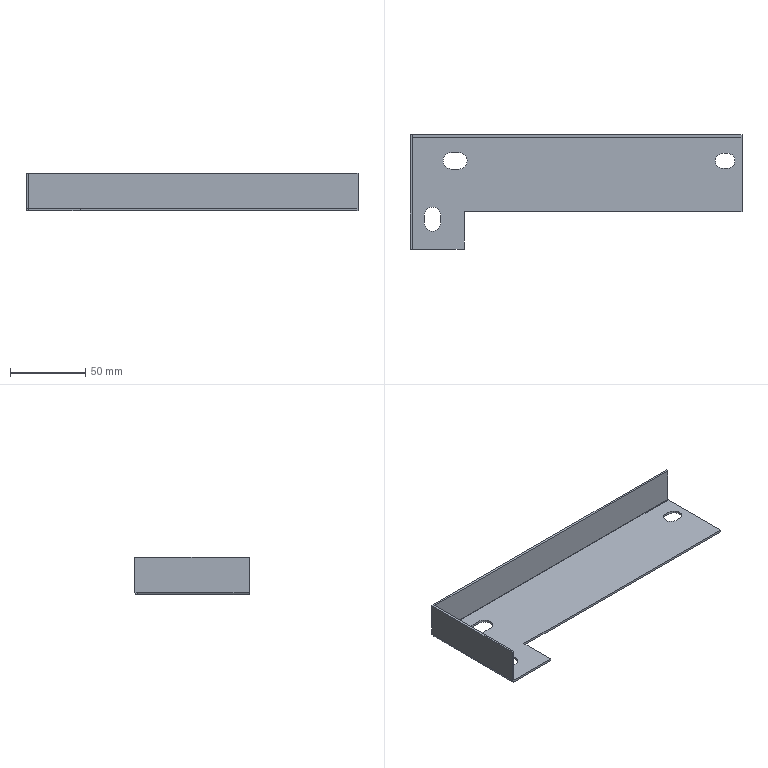Part | SolidWorks | features Cut 5, EdgeFlange 3, ICE 2, FlatPattern 1, MirrorPattern 1, SMBaseFlange 1, SheetMetal 1 | 1 solid | 39 faces | box 221 x 76 x 25 mm | volume 27869 mm3 | plane 27 | cylinder 12 | commonest cylinder face diameters 11 x5 10 x3 0.4 x2 3.4 x2
STEP:
#1=CARTESIAN_POINT('',(105.8,20.8,-1.5));
#2=VERTEX_POINT('',#1);
#3=CARTESIAN_POINT('',(100.8,25.8,-1.5));
#4=VERTEX_POINT('',#3);
#5=CARTESIAN_POINT('',(100.8,20.8,-1.5));
#6=DIRECTION('',(0.,0.,1.));
#7=DIRECTION('',(1.,0.,0.));
#8=AXIS2_PLACEMENT_3D('',#5,#6,#7);
#9=CIRCLE('',#8,5.);
#10=EDGE_CURVE('',#2,#4,#9,.T.);
#11=ORIENTED_EDGE('',*,*,#10,.F.);
#12=CARTESIAN_POINT('',(105.8,20.8,0.));
#13=VERTEX_POINT('',#12);
#14=CARTESIAN_POINT('',(105.8,20.8,-10.));
#15=DIRECTION('',(0.,0.,1.));
#16=VECTOR('',#15,1000.);
#17=LINE('',#14,#16);
#18=EDGE_CURVE('',#2,#13,#17,.T.);
#19=ORIENTED_EDGE('',*,*,#18,.T.);
#20=CARTESIAN_POINT('',(100.8,25.8,0.));
#21=VERTEX_POINT('',#20);
#22=CARTESIAN_POINT('',(100.8,20.8,0.));
#23=DIRECTION('',(0.,0.,1.));
#24=DIRECTION('',(1.,0.,0.));
#25=AXIS2_PLACEMENT_3D('',#22,#23,#24);
#26=CIRCLE('',#25,5.);
#27=EDGE_CURVE('',#13,#21,#26,.T.);
#28=ORIENTED_EDGE('',*,*,#27,.T.);
#29=CARTESIAN_POINT('',(100.8,25.8,-10.));
#30=DIRECTION('',(0.,0.,1.));
#31=VECTOR('',#30,1000.);
#32=LINE('',#29,#31);
#33=EDGE_CURVE('',#4,#21,#32,.T.);
#34=ORIENTED_EDGE('',*,*,#33,.F.);
#35=EDGE_LOOP('',(#11,#19,#28,#34));
#36=FACE_OUTER_BOUND('',#35,.T.);
#37=CARTESIAN_POINT('',(100.8,20.8,-10.));
#38=DIRECTION('',(0.,0.,1.));
#39=DIRECTION('',(1.,0.,0.));
#40=AXIS2_PLACEMENT_3D('',#37,#38,#39);
#41=CYLINDRICAL_SURFACE('',#40,5.);
#42=ADVANCED_FACE('',(#36),#41,.F.);
#43=CARTESIAN_POINT('',(-72.5,20.8,-1.5));
#44=VERTEX_POINT('',#43);
#45=CARTESIAN_POINT('',(-78.,26.3,-1.5));
#46=VERTEX_POINT('',#45);
#47=CARTESIAN_POINT('',(-78.,20.8,-1.5));
#48=DIRECTION('',(0.,0.,1.));
#49=DIRECTION('',(1.,0.,0.));
#50=AXIS2_PLACEMENT_3D('',#47,#48,#49);
#51=CIRCLE('',#50,5.5);
#52=EDGE_CURVE('',#44,#46,#51,.T.);
#53=ORIENTED_EDGE('',*,*,#52,.F.);
#54=CARTESIAN_POINT('',(-72.5,20.8,0.));
#55=VERTEX_POINT('',#54);
#56=CARTESIAN_POINT('',(-72.5,20.8,-10.));
#57=DIRECTION('',(0.,0.,1.));
#58=VECTOR('',#57,1000.);
#59=LINE('',#56,#58);
#60=EDGE_CURVE('',#44,#55,#59,.T.);
#61=ORIENTED_EDGE('',*,*,#60,.T.);
#62=CARTESIAN_POINT('',(-78.,26.3,0.));
#63=VERTEX_POINT('',#62);
#64=CARTESIAN_POINT('',(-78.,20.8,0.));
#65=DIRECTION('',(0.,0.,1.));
#66=DIRECTION('',(1.,0.,0.));
#67=AXIS2_PLACEMENT_3D('',#64,#65,#66);
#68=CIRCLE('',#67,5.5);
#69=EDGE_CURVE('',#55,#63,#68,.T.);
#70=ORIENTED_EDGE('',*,*,#69,.T.);
#71=CARTESIAN_POINT('',(-78.,26.3,-10.));
#72=DIRECTION('',(0.,0.,1.));
#73=VECTOR('',#72,1000.);
#74=LINE('',#71,#73);
#75=EDGE_CURVE('',#46,#63,#74,.T.);
#76=ORIENTED_EDGE('',*,*,#75,.F.);
#77=EDGE_LOOP('',(#53,#61,#70,#76));
#78=FACE_OUTER_BOUND('',#77,.T.);
#79=CARTESIAN_POINT('',(-78.,20.8,-10.));
#80=DIRECTION('',(0.,0.,1.));
#81=DIRECTION('',(1.,0.,0.));
#82=AXIS2_PLACEMENT_3D('',#79,#80,#81);
#83=CYLINDRICAL_SURFACE('',#82,5.5);
#84=ADVANCED_FACE('',(#78),#83,.F.);
#85=CARTESIAN_POINT('',(-110.5,36.3,0.2));
#86=VERTEX_POINT('',#85);
#87=CARTESIAN_POINT('',(-109.,36.3,0.2));
#88=VERTEX_POINT('',#87);
#89=CARTESIAN_POINT('',(-110.5,36.3,0.2));
#90=DIRECTION('',(1.,0.,0.));
#91=VECTOR('',#90,1000.);
#92=LINE('',#89,#91);
#93=EDGE_CURVE('',#86,#88,#92,.T.);
#94=ORIENTED_EDGE('',*,*,#93,.F.);
#95=CARTESIAN_POINT('',(-110.5,38.,0.2));
#96=VERTEX_POINT('',#95);
#97=CARTESIAN_POINT('',(-110.5,38.,0.2));
#98=DIRECTION('',(0.,1.,0.));
#99=VECTOR('',#98,1000.);
#100=LINE('',#97,#99);
#101=EDGE_CURVE('',#86,#96,#100,.T.);
#102=ORIENTED_EDGE('',*,*,#101,.T.);
#103=CARTESIAN_POINT('',(-109.,38.,0.2));
#104=VERTEX_POINT('',#103);
#105=CARTESIAN_POINT('',(-110.5,38.,0.2));
#106=DIRECTION('',(-1.,0.,0.));
#107=VECTOR('',#106,1000.);
#108=LINE('',#105,#107);
#109=EDGE_CURVE('',#104,#96,#108,.T.);
#110=ORIENTED_EDGE('',*,*,#109,.F.);
#111=CARTESIAN_POINT('',(-109.,38.,0.2));
#112=DIRECTION('',(0.,-1.,0.));
#113=VECTOR('',#112,1000.);
#114=LINE('',#111,#113);
#115=EDGE_CURVE('',#104,#88,#114,.T.);
#116=ORIENTED_EDGE('',*,*,#115,.T.);
#117=EDGE_LOOP('',(#94,#102,#110,#116));
#118=FACE_OUTER_BOUND('',#117,.T.);
#119=CARTESIAN_POINT('',(0.,0.,0.2));
#120=DIRECTION('',(0.,0.,-1.));
#121=DIRECTION('',(-1.,0.,0.));
#122=AXIS2_PLACEMENT_3D('',#119,#120,#121);
#123=PLANE('',#122);
#124=ADVANCED_FACE('',(#118),#123,.T.);
#125=CARTESIAN_POINT('',(-110.5,-38.,0.2));
#126=VERTEX_POINT('',#125);
#127=CARTESIAN_POINT('',(-110.5,38.,0.2));
#128=DIRECTION('',(0.,1.,0.));
#129=VECTOR('',#128,1000.);
#130=LINE('',#127,#129);
#131=EDGE_CURVE('',#126,#86,#130,.T.);
#132=ORIENTED_EDGE('',*,*,#131,.T.);
#133=CARTESIAN_POINT('',(-108.8,36.3,-1.5));
#134=VERTEX_POINT('',#133);
#135=CARTESIAN_POINT('',(-108.8,36.3,0.2));
#136=DIRECTION('',(0.,-1.,0.));
#137=DIRECTION('',(0.,0.,1.));
#138=AXIS2_PLACEMENT_3D('',#135,#136,#137);
#139=CIRCLE('',#138,1.7);
#140=EDGE_CURVE('',#86,#134,#139,.T.);
#141=ORIENTED_EDGE('',*,*,#140,.T.);
#142=CARTESIAN_POINT('',(-108.8,-38.,-1.5));
#143=VERTEX_POINT('',#142);
#144=CARTESIAN_POINT('',(-108.8,-38.,-1.5));
#145=DIRECTION('',(0.,1.,0.));
#146=VECTOR('',#145,1000.);
#147=LINE('',#144,#146);
#148=EDGE_CURVE('',#143,#134,#147,.T.);
#149=ORIENTED_EDGE('',*,*,#148,.F.);
#150=CARTESIAN_POINT('',(-108.8,-38.,0.2));
#151=DIRECTION('',(0.,-1.,0.));
#152=DIRECTION('',(0.,0.,-1.));
#153=AXIS2_PLACEMENT_3D('',#150,#151,#152);
#154=CIRCLE('',#153,1.7);
#155=EDGE_CURVE('',#126,#143,#154,.T.);
#156=ORIENTED_EDGE('',*,*,#155,.F.);
#157=EDGE_LOOP('',(#132,#141,#149,#156));
#158=FACE_OUTER_BOUND('',#157,.T.);
#159=CARTESIAN_POINT('',(-108.8,-38.,0.2));
#160=DIRECTION('',(0.,-1.,0.));
#161=DIRECTION('',(-1.,0.,0.));
#162=AXIS2_PLACEMENT_3D('',#159,#160,#161);
#163=CYLINDRICAL_SURFACE('',#162,1.7);
#164=ADVANCED_FACE('',(#158),#163,.T.);
#165=CARTESIAN_POINT('',(97.8,25.8,-1.5));
#166=VERTEX_POINT('',#165);
#167=CARTESIAN_POINT('',(0.,25.8,-1.5));
#168=DIRECTION('',(-1.,0.,0.));
#169=VECTOR('',#168,1000.);
#170=LINE('',#167,#169);
#171=EDGE_CURVE('',#4,#166,#170,.T.);
#172=ORIENTED_EDGE('',*,*,#171,.T.);
#173=CARTESIAN_POINT('',(97.8,15.8,-1.5));
#174=VERTEX_POINT('',#173);
#175=CARTESIAN_POINT('',(97.8,20.8,-1.5));
#176=DIRECTION('',(0.,0.,1.));
#177=DIRECTION('',(1.,0.,0.));
#178=AXIS2_PLACEMENT_3D('',#175,#176,#177);
#179=CIRCLE('',#178,5.);
#180=EDGE_CURVE('',#166,#174,#179,.T.);
#181=ORIENTED_EDGE('',*,*,#180,.T.);
#182=CARTESIAN_POINT('',(100.8,15.8,-1.5));
#183=VERTEX_POINT('',#182);
#184=CARTESIAN_POINT('',(0.,15.8,-1.5));
#185=DIRECTION('',(1.,0.,0.));
#186=VECTOR('',#185,1000.);
#187=LINE('',#184,#186);
#188=EDGE_CURVE('',#174,#183,#187,.T.);
#189=ORIENTED_EDGE('',*,*,#188,.T.);
#190=CARTESIAN_POINT('',(100.8,20.8,-1.5));
#191=DIRECTION('',(0.,0.,1.));
#192=DIRECTION('',(1.,0.,0.));
#193=AXIS2_PLACEMENT_3D('',#190,#191,#192);
#194=CIRCLE('',#193,5.);
#195=EDGE_CURVE('',#183,#2,#194,.T.);
#196=ORIENTED_EDGE('',*,*,#195,.T.);
#197=ORIENTED_EDGE('',*,*,#10,.T.);
#198=EDGE_LOOP('',(#172,#181,#189,#196,#197));
#199=FACE_BOUND('',#198,.T.);
#200=CARTESIAN_POINT('',(-83.,26.3,-1.5));
#201=VERTEX_POINT('',#200);
#202=CARTESIAN_POINT('',(0.,26.3,-1.5));
#203=DIRECTION('',(-1.,0.,0.));
#204=VECTOR('',#203,1000.);
#205=LINE('',#202,#204);
#206=EDGE_CURVE('',#46,#201,#205,.T.);
#207=ORIENTED_EDGE('',*,*,#206,.T.);
#208=CARTESIAN_POINT('',(-83.,15.3,-1.5));
#209=VERTEX_POINT('',#208);
#210=CARTESIAN_POINT('',(-83.,20.8,-1.5));
#211=DIRECTION('',(0.,0.,1.));
#212=DIRECTION('',(1.,0.,0.));
#213=AXIS2_PLACEMENT_3D('',#210,#211,#212);
#214=CIRCLE('',#213,5.5);
#215=EDGE_CURVE('',#201,#209,#214,.T.);
#216=ORIENTED_EDGE('',*,*,#215,.T.);
#217=CARTESIAN_POINT('',(-78.,15.3,-1.5));
#218=VERTEX_POINT('',#217);
#219=CARTESIAN_POINT('',(0.,15.3,-1.5));
#220=DIRECTION('',(1.,0.,0.));
#221=VECTOR('',#220,1000.);
#222=LINE('',#219,#221);
#223=EDGE_CURVE('',#209,#218,#222,.T.);
#224=ORIENTED_EDGE('',*,*,#223,.T.);
#225=CARTESIAN_POINT('',(-78.,20.8,-1.5));
#226=DIRECTION('',(0.,0.,1.));
#227=DIRECTION('',(1.,0.,0.));
#228=AXIS2_PLACEMENT_3D('',#225,#226,#227);
#229=CIRCLE('',#228,5.5);
#230=EDGE_CURVE('',#218,#44,#229,.T.);
#231=ORIENTED_EDGE('',*,*,#230,.T.);
#232=ORIENTED_EDGE('',*,*,#52,.T.);
#233=EDGE_LOOP('',(#207,#216,#224,#231,#232));
#234=FACE_BOUND('',#233,.T.);
#235=CARTESIAN_POINT('',(-90.,-20.5,-1.5));
#236=VERTEX_POINT('',#235);
#237=CARTESIAN_POINT('',(-90.,-15.5,-1.5));
#238=VERTEX_POINT('',#237);
#239=CARTESIAN_POINT('',(-90.,0.,-1.5));
#240=DIRECTION('',(0.,1.,0.));
#241=VECTOR('',#240,1000.);
#242=LINE('',#239,#241);
#243=EDGE_CURVE('',#236,#238,#242,.T.);
#244=ORIENTED_EDGE('',*,*,#243,.T.);
#245=CARTESIAN_POINT('',(-101.,-15.5,-1.5));
#246=VERTEX_POINT('',#245);
#247=CARTESIAN_POINT('',(-95.5,-15.5,-1.5));
#248=DIRECTION('',(0.,0.,1.));
#249=DIRECTION('',(1.,0.,0.));
#250=AXIS2_PLACEMENT_3D('',#247,#248,#249);
#251=CIRCLE('',#250,5.5);
#252=EDGE_CURVE('',#238,#246,#251,.T.);
#253=ORIENTED_EDGE('',*,*,#252,.T.);
#254=CARTESIAN_POINT('',(-101.,-20.5,-1.5));
#255=VERTEX_POINT('',#254);
#256=CARTESIAN_POINT('',(-101.,0.,-1.5));
#257=DIRECTION('',(0.,-1.,0.));
#258=VECTOR('',#257,1000.);
#259=LINE('',#256,#258);
#260=EDGE_CURVE('',#246,#255,#259,.T.);
#261=ORIENTED_EDGE('',*,*,#260,.T.);
#262=CARTESIAN_POINT('',(-95.5,-20.5,-1.5));
#263=DIRECTION('',(0.,0.,1.));
#264=DIRECTION('',(1.,0.,0.));
#265=AXIS2_PLACEMENT_3D('',#262,#263,#264);
#266=CIRCLE('',#265,5.5);
#267=EDGE_CURVE('',#255,#236,#266,.T.);
#268=ORIENTED_EDGE('',*,*,#267,.T.);
#269=EDGE_LOOP('',(#244,#253,#261,#268));
#270=FACE_BOUND('',#269,.T.);
#271=CARTESIAN_POINT('',(110.5,-13.,-1.5));
#272=VERTEX_POINT('',#271);
#273=CARTESIAN_POINT('',(110.5,36.3,-1.5));
#274=VERTEX_POINT('',#273);
#275=CARTESIAN_POINT('',(110.5,38.,-1.5));
#276=DIRECTION('',(0.,1.,0.));
#277=VECTOR('',#276,1000.);
#278=LINE('',#275,#277);
#279=EDGE_CURVE('',#272,#274,#278,.T.);
#280=ORIENTED_EDGE('',*,*,#279,.F.);
#281=CARTESIAN_POINT('',(-74.5,-13.,-1.5));
#282=VERTEX_POINT('',#281);
#283=CARTESIAN_POINT('',(110.5,-13.,-1.5));
#284=DIRECTION('',(1.,0.,0.));
#285=VECTOR('',#284,1000.);
#286=LINE('',#283,#285);
#287=EDGE_CURVE('',#282,#272,#286,.T.);
#288=ORIENTED_EDGE('',*,*,#287,.F.);
#289=CARTESIAN_POINT('',(-74.5,-38.,-1.5));
#290=VERTEX_POINT('',#289);
#291=CARTESIAN_POINT('',(-74.5,-38.,-1.5));
#292=DIRECTION('',(0.,1.,0.));
#293=VECTOR('',#292,1000.);
#294=LINE('',#291,#293);
#295=EDGE_CURVE('',#290,#282,#294,.T.);
#296=ORIENTED_EDGE('',*,*,#295,.F.);
#297=CARTESIAN_POINT('',(-110.5,-38.,-1.5));
#298=DIRECTION('',(1.,0.,0.));
#299=VECTOR('',#298,1000.);
#300=LINE('',#297,#299);
#301=EDGE_CURVE('',#143,#290,#300,.T.);
#302=ORIENTED_EDGE('',*,*,#301,.F.);
#303=ORIENTED_EDGE('',*,*,#148,.T.);
#304=CARTESIAN_POINT('',(-108.8,36.3,-1.5));
#305=DIRECTION('',(1.,0.,0.));
#306=VECTOR('',#305,1000.);
#307=LINE('',#304,#306);
#308=EDGE_CURVE('',#134,#274,#307,.T.);
#309=ORIENTED_EDGE('',*,*,#308,.T.);
#310=EDGE_LOOP('',(#280,#288,#296,#302,#303,#309));
#311=FACE_OUTER_BOUND('',#310,.T.);
#312=CARTESIAN_POINT('',(0.,0.,-1.5));
#313=DIRECTION('',(0.,0.,1.));
#314=DIRECTION('',(1.,0.,0.));
#315=AXIS2_PLACEMENT_3D('',#312,#313,#314);
#316=PLANE('',#315);
#317=ADVANCED_FACE('',(#199,#234,#270,#311),#316,.F.);
#318=CARTESIAN_POINT('',(110.5,-13.,0.));
#319=VERTEX_POINT('',#318);
#320=CARTESIAN_POINT('',(-74.5,-13.,0.));
#321=VERTEX_POINT('',#320);
#322=CARTESIAN_POINT('',(0.,-13.,0.));
#323=DIRECTION('',(-1.,0.,0.));
#324=VECTOR('',#323,1000.);
#325=LINE('',#322,#324);
#326=EDGE_CURVE('',#319,#321,#325,.T.);
#327=ORIENTED_EDGE('',*,*,#326,.F.);
#328=CARTESIAN_POINT('',(110.5,36.3,0.));
#329=VERTEX_POINT('',#328);
#330=CARTESIAN_POINT('',(110.5,38.,0.));
#331=DIRECTION('',(0.,1.,0.));
#332=VECTOR('',#331,1000.);
#333=LINE('',#330,#332);
#334=EDGE_CURVE('',#319,#329,#333,.T.);
#335=ORIENTED_EDGE('',*,*,#334,.T.);
#336=CARTESIAN_POINT('',(-108.8,36.3,0.));
#337=VERTEX_POINT('',#336);
#338=CARTESIAN_POINT('',(-108.8,36.3,0.));
#339=DIRECTION('',(1.,0.,0.));
#340=VECTOR('',#339,1000.);
#341=LINE('',#338,#340);
#342=EDGE_CURVE('',#337,#329,#341,.T.);
#343=ORIENTED_EDGE('',*,*,#342,.F.);
#344=CARTESIAN_POINT('',(-108.8,-38.,0.));
#345=VERTEX_POINT('',#344);
#346=CARTESIAN_POINT('',(-108.8,-38.,0.));
#347=DIRECTION('',(0.,1.,0.));
#348=VECTOR('',#347,1000.);
#349=LINE('',#346,#348);
#350=EDGE_CURVE('',#345,#337,#349,.T.);
#351=ORIENTED_EDGE('',*,*,#350,.F.);
#352=CARTESIAN_POINT('',(-74.5,-38.,0.));
#353=VERTEX_POINT('',#352);
#354=CARTESIAN_POINT('',(-110.5,-38.,0.));
#355=DIRECTION('',(1.,0.,0.));
#356=VECTOR('',#355,1000.);
#357=LINE('',#354,#356);
#358=EDGE_CURVE('',#345,#353,#357,.T.);
#359=ORIENTED_EDGE('',*,*,#358,.T.);
#360=CARTESIAN_POINT('',(-74.5,0.,0.));
#361=DIRECTION('',(0.,-1.,0.));
#362=VECTOR('',#361,1000.);
#363=LINE('',#360,#362);
#364=EDGE_CURVE('',#321,#353,#363,.T.);
#365=ORIENTED_EDGE('',*,*,#364,.F.);
#366=EDGE_LOOP('',(#327,#335,#343,#351,#359,#365));
#367=FACE_OUTER_BOUND('',#366,.T.);
#368=CARTESIAN_POINT('',(97.8,25.8,0.));
#369=VERTEX_POINT('',#368);
#370=CARTESIAN_POINT('',(97.8,15.8,0.));
#371=VERTEX_POINT('',#370);
#372=CARTESIAN_POINT('',(97.8,20.8,0.));
#373=DIRECTION('',(0.,0.,1.));
#374=DIRECTION('',(1.,0.,0.));
#375=AXIS2_PLACEMENT_3D('',#372,#373,#374);
#376=CIRCLE('',#375,5.);
#377=EDGE_CURVE('',#369,#371,#376,.T.);
#378=ORIENTED_EDGE('',*,*,#377,.F.);
#379=CARTESIAN_POINT('',(97.8,25.8,0.));
#380=DIRECTION('',(-1.,0.,0.));
#381=VECTOR('',#380,1000.);
#382=LINE('',#379,#381);
#383=EDGE_CURVE('',#21,#369,#382,.T.);
#384=ORIENTED_EDGE('',*,*,#383,.F.);
#385=ORIENTED_EDGE('',*,*,#27,.F.);
#386=CARTESIAN_POINT('',(100.8,15.8,0.));
#387=VERTEX_POINT('',#386);
#388=CARTESIAN_POINT('',(100.8,20.8,0.));
#389=DIRECTION('',(0.,0.,1.));
#390=DIRECTION('',(1.,0.,0.));
#391=AXIS2_PLACEMENT_3D('',#388,#389,#390);
#392=CIRCLE('',#391,5.);
#393=EDGE_CURVE('',#387,#13,#392,.T.);
#394=ORIENTED_EDGE('',*,*,#393,.F.);
#395=CARTESIAN_POINT('',(97.8,15.8,0.));
#396=DIRECTION('',(1.,0.,0.));
#397=VECTOR('',#396,1000.);
#398=LINE('',#395,#397);
#399=EDGE_CURVE('',#371,#387,#398,.T.);
#400=ORIENTED_EDGE('',*,*,#399,.F.);
#401=EDGE_LOOP('',(#378,#384,#385,#394,#400));
#402=FACE_BOUND('',#401,.T.);
#403=CARTESIAN_POINT('',(-83.,26.3,0.));
#404=VERTEX_POINT('',#403);
#405=CARTESIAN_POINT('',(-83.,15.3,0.));
#406=VERTEX_POINT('',#405);
#407=CARTESIAN_POINT('',(-83.,20.8,0.));
#408=DIRECTION('',(0.,0.,1.));
#409=DIRECTION('',(1.,0.,0.));
#410=AXIS2_PLACEMENT_3D('',#407,#408,#409);
#411=CIRCLE('',#410,5.5);
#412=EDGE_CURVE('',#404,#406,#411,.T.);
#413=ORIENTED_EDGE('',*,*,#412,.F.);
#414=CARTESIAN_POINT('',(-83.,26.3,0.));
#415=DIRECTION('',(-1.,0.,0.));
#416=VECTOR('',#415,1000.);
#417=LINE('',#414,#416);
#418=EDGE_CURVE('',#63,#404,#417,.T.);
#419=ORIENTED_EDGE('',*,*,#418,.F.);
#420=ORIENTED_EDGE('',*,*,#69,.F.);
#421=CARTESIAN_POINT('',(-78.,15.3,0.));
#422=VERTEX_POINT('',#421);
#423=CARTESIAN_POINT('',(-78.,20.8,0.));
#424=DIRECTION('',(0.,0.,1.));
#425=DIRECTION('',(1.,0.,0.));
#426=AXIS2_PLACEMENT_3D('',#423,#424,#425);
#427=CIRCLE('',#426,5.5);
#428=EDGE_CURVE('',#422,#55,#427,.T.);
#429=ORIENTED_EDGE('',*,*,#428,.F.);
#430=CARTESIAN_POINT('',(-83.,15.3,0.));
#431=DIRECTION('',(1.,0.,0.));
#432=VECTOR('',#431,1000.);
#433=LINE('',#430,#432);
#434=EDGE_CURVE('',#406,#422,#433,.T.);
#435=ORIENTED_EDGE('',*,*,#434,.F.);
#436=EDGE_LOOP('',(#413,#419,#420,#429,#435));
#437=FACE_BOUND('',#436,.T.);
#438=CARTESIAN_POINT('',(-90.,-15.5,0.));
#439=VERTEX_POINT('',#438);
#440=CARTESIAN_POINT('',(-101.,-15.5,0.));
#441=VERTEX_POINT('',#440);
#442=CARTESIAN_POINT('',(-95.5,-15.5,0.));
#443=DIRECTION('',(0.,0.,1.));
#444=DIRECTION('',(1.,0.,0.));
#445=AXIS2_PLACEMENT_3D('',#442,#443,#444);
#446=CIRCLE('',#445,5.5);
#447=EDGE_CURVE('',#439,#441,#446,.T.);
#448=ORIENTED_EDGE('',*,*,#447,.F.);
#449=CARTESIAN_POINT('',(-90.,-20.5,0.));
#450=VERTEX_POINT('',#449);
#451=CARTESIAN_POINT('',(-90.,-15.5,0.));
#452=DIRECTION('',(0.,1.,0.));
#453=VECTOR('',#452,1000.);
#454=LINE('',#451,#453);
#455=EDGE_CURVE('',#450,#439,#454,.T.);
#456=ORIENTED_EDGE('',*,*,#455,.F.);
#457=CARTESIAN_POINT('',(-101.,-20.5,0.));
#458=VERTEX_POINT('',#457);
#459=CARTESIAN_POINT('',(-95.5,-20.5,0.));
#460=DIRECTION('',(0.,0.,1.));
#461=DIRECTION('',(1.,0.,0.));
#462=AXIS2_PLACEMENT_3D('',#459,#460,#461);
#463=CIRCLE('',#462,5.5);
#464=EDGE_CURVE('',#458,#450,#463,.T.);
#465=ORIENTED_EDGE('',*,*,#464,.F.);
#466=CARTESIAN_POINT('',(-101.,-15.5,0.));
#467=DIRECTION('',(0.,-1.,0.));
#468=VECTOR('',#467,1000.);
#469=LINE('',#466,#468);
#470=EDGE_CURVE('',#441,#458,#469,.T.);
#471=ORIENTED_EDGE('',*,*,#470,.F.);
#472=EDGE_LOOP('',(#448,#456,#465,#471));
#473=FACE_BOUND('',#472,.T.);
#474=CARTESIAN_POINT('',(0.,0.,0.));
#475=DIRECTION('',(0.,0.,1.));
#476=DIRECTION('',(1.,0.,0.));
#477=AXIS2_PLACEMENT_3D('',#474,#475,#476);
#478=PLANE('',#477);
#479=ADVANCED_FACE('',(#367,#402,#437,#473),#478,.T.);
#480=CARTESIAN_POINT('',(-74.5,-38.,8.5));
#481=DIRECTION('',(0.,0.,-1.));
#482=VECTOR('',#481,1000.);
#483=LINE('',#480,#482);
#484=EDGE_CURVE('',#353,#290,#483,.T.);
#485=ORIENTED_EDGE('',*,*,#484,.F.);
#486=ORIENTED_EDGE('',*,*,#358,.F.);
#487=CARTESIAN_POINT('',(-108.8,-38.,0.));
#488=DIRECTION('',(0.,0.,-1.));
#489=VECTOR('',#488,1000.);
#490=LINE('',#487,#489);
#491=EDGE_CURVE('',#345,#143,#490,.T.);
#492=ORIENTED_EDGE('',*,*,#491,.T.);
#493=ORIENTED_EDGE('',*,*,#301,.T.);
#494=EDGE_LOOP('',(#485,#486,#492,#493));
#495=FACE_OUTER_BOUND('',#494,.T.);
#496=CARTESIAN_POINT('',(-110.5,-38.,-1.5));
#497=DIRECTION('',(0.,-1.,0.));
#498=DIRECTION('',(0.,0.,-1.));
#499=AXIS2_PLACEMENT_3D('',#496,#497,#498);
#500=PLANE('',#499);
#501=ADVANCED_FACE('',(#495),#500,.T.);
#502=CARTESIAN_POINT('',(110.5,-13.,-1.5));
#503=DIRECTION('',(0.,0.,1.));
#504=VECTOR('',#503,1000.);
#505=LINE('',#502,#504);
#506=EDGE_CURVE('',#272,#319,#505,.T.);
#507=ORIENTED_EDGE('',*,*,#506,.F.);
#508=ORIENTED_EDGE('',*,*,#279,.T.);
#509=CARTESIAN_POINT('',(110.5,36.3,0.));
#510=DIRECTION('',(0.,0.,-1.));
#511=VECTOR('',#510,1000.);
#512=LINE('',#509,#511);
#513=EDGE_CURVE('',#329,#274,#512,.T.);
#514=ORIENTED_EDGE('',*,*,#513,.F.);
#515=ORIENTED_EDGE('',*,*,#334,.F.);
#516=EDGE_LOOP('',(#507,#508,#514,#515));
#517=FACE_OUTER_BOUND('',#516,.T.);
#518=CARTESIAN_POINT('',(110.5,38.,-1.5));
#519=DIRECTION('',(1.,0.,0.));
#520=DIRECTION('',(0.,0.,-1.));
#521=AXIS2_PLACEMENT_3D('',#518,#519,#520);
#522=PLANE('',#521);
#523=ADVANCED_FACE('',(#517),#522,.T.);
#524=CARTESIAN_POINT('',(-90.,-15.5,-10.));
#525=DIRECTION('',(0.,0.,1.));
#526=VECTOR('',#525,1000.);
#527=LINE('',#524,#526);
#528=EDGE_CURVE('',#238,#439,#527,.T.);
#529=ORIENTED_EDGE('',*,*,#528,.T.);
#530=ORIENTED_EDGE('',*,*,#447,.T.);
#531=CARTESIAN_POINT('',(-101.,-15.5,-10.));
#532=DIRECTION('',(0.,0.,1.));
#533=VECTOR('',#532,1000.);
#534=LINE('',#531,#533);
#535=EDGE_CURVE('',#246,#441,#534,.T.);
#536=ORIENTED_EDGE('',*,*,#535,.F.);
#537=ORIENTED_EDGE('',*,*,#252,.F.);
#538=EDGE_LOOP('',(#529,#530,#536,#537));
#539=FACE_OUTER_BOUND('',#538,.T.);
#540=CARTESIAN_POINT('',(-95.5,-15.5,-10.));
#541=DIRECTION('',(0.,0.,1.));
#542=DIRECTION('',(1.,0.,0.));
#543=AXIS2_PLACEMENT_3D('',#540,#541,#542);
#544=CYLINDRICAL_SURFACE('',#543,5.5);
#545=ADVANCED_FACE('',(#539),#544,.F.);
#546=CARTESIAN_POINT('',(-90.,-20.5,-10.));
#547=DIRECTION('',(0.,0.,1.));
#548=VECTOR('',#547,1000.);
#549=LINE('',#546,#548);
#550=EDGE_CURVE('',#236,#450,#549,.T.);
#551=ORIENTED_EDGE('',*,*,#550,.T.);
#552=ORIENTED_EDGE('',*,*,#455,.T.);
#553=ORIENTED_EDGE('',*,*,#528,.F.);
#554=ORIENTED_EDGE('',*,*,#243,.F.);
#555=EDGE_LOOP('',(#551,#552,#553,#554));
#556=FACE_OUTER_BOUND('',#555,.T.);
#557=CARTESIAN_POINT('',(-90.,-15.5,-10.));
#558=DIRECTION('',(1.,0.,0.));
#559=DIRECTION('',(0.,0.,-1.));
#560=AXIS2_PLACEMENT_3D('',#557,#558,#559);
#561=PLANE('',#560);
#562=ADVANCED_FACE('',(#556),#561,.F.);
#563=CARTESIAN_POINT('',(-101.,-20.5,-10.));
#564=DIRECTION('',(0.,0.,1.));
#565=VECTOR('',#564,1000.);
#566=LINE('',#563,#565);
#567=EDGE_CURVE('',#255,#458,#566,.T.);
#568=ORIENTED_EDGE('',*,*,#567,.T.);
#569=ORIENTED_EDGE('',*,*,#464,.T.);
#570=ORIENTED_EDGE('',*,*,#550,.F.);
#571=ORIENTED_EDGE('',*,*,#267,.F.);
#572=EDGE_LOOP('',(#568,#569,#570,#571));
#573=FACE_OUTER_BOUND('',#572,.T.);
#574=CARTESIAN_POINT('',(-95.5,-20.5,-10.));
#575=DIRECTION('',(0.,0.,1.));
#576=DIRECTION('',(1.,0.,0.));
#577=AXIS2_PLACEMENT_3D('',#574,#575,#576);
#578=CYLINDRICAL_SURFACE('',#577,5.5);
#579=ADVANCED_FACE('',(#573),#578,.F.);
#580=ORIENTED_EDGE('',*,*,#535,.T.);
#581=ORIENTED_EDGE('',*,*,#470,.T.);
#582=ORIENTED_EDGE('',*,*,#567,.F.);
#583=ORIENTED_EDGE('',*,*,#260,.F.);
#584=EDGE_LOOP('',(#580,#581,#582,#583));
#585=FACE_OUTER_BOUND('',#584,.T.);
#586=CARTESIAN_POINT('',(-101.,-15.5,-10.));
#587=DIRECTION('',(-1.,0.,0.));
#588=DIRECTION('',(0.,0.,1.));
#589=AXIS2_PLACEMENT_3D('',#586,#587,#588);
#590=PLANE('',#589);
#591=ADVANCED_FACE('',(#585),#590,.F.);
#592=CARTESIAN_POINT('',(-83.,26.3,-10.));
#593=DIRECTION('',(0.,0.,1.));
#594=VECTOR('',#593,1000.);
#595=LINE('',#592,#594);
#596=EDGE_CURVE('',#201,#404,#595,.T.);
#597=ORIENTED_EDGE('',*,*,#596,.T.);
#598=ORIENTED_EDGE('',*,*,#412,.T.);
#599=CARTESIAN_POINT('',(-83.,15.3,-10.));
#600=DIRECTION('',(0.,0.,1.));
#601=VECTOR('',#600,1000.);
#602=LINE('',#599,#601);
#603=EDGE_CURVE('',#209,#406,#602,.T.);
#604=ORIENTED_EDGE('',*,*,#603,.F.);
#605=ORIENTED_EDGE('',*,*,#215,.F.);
#606=EDGE_LOOP('',(#597,#598,#604,#605));
#607=FACE_OUTER_BOUND('',#606,.T.);
#608=CARTESIAN_POINT('',(-83.,20.8,-10.));
#609=DIRECTION('',(0.,0.,1.));
#610=DIRECTION('',(1.,0.,0.));
#611=AXIS2_PLACEMENT_3D('',#608,#609,#610);
#612=CYLINDRICAL_SURFACE('',#611,5.5);
#613=ADVANCED_FACE('',(#607),#612,.F.);
#614=ORIENTED_EDGE('',*,*,#75,.T.);
#615=ORIENTED_EDGE('',*,*,#418,.T.);
#616=ORIENTED_EDGE('',*,*,#596,.F.);
#617=ORIENTED_EDGE('',*,*,#206,.F.);
#618=EDGE_LOOP('',(#614,#615,#616,#617));
#619=FACE_OUTER_BOUND('',#618,.T.);
#620=CARTESIAN_POINT('',(-83.,26.3,-10.));
#621=DIRECTION('',(0.,1.,0.));
#622=DIRECTION('',(0.,0.,1.));
#623=AXIS2_PLACEMENT_3D('',#620,#621,#622);
#624=PLANE('',#623);
#625=ADVANCED_FACE('',(#619),#624,.F.);
#626=ORIENTED_EDGE('',*,*,#60,.F.);
#627=ORIENTED_EDGE('',*,*,#230,.F.);
#628=CARTESIAN_POINT('',(-78.,15.3,-10.));
#629=DIRECTION('',(0.,0.,1.));
#630=VECTOR('',#629,1000.);
#631=LINE('',#628,#630);
#632=EDGE_CURVE('',#218,#422,#631,.T.);
#633=ORIENTED_EDGE('',*,*,#632,.T.);
#634=ORIENTED_EDGE('',*,*,#428,.T.);
#635=EDGE_LOOP('',(#626,#627,#633,#634));
#636=FACE_OUTER_BOUND('',#635,.T.);
#637=CARTESIAN_POINT('',(-78.,20.8,-10.));
#638=DIRECTION('',(0.,0.,1.));
#639=DIRECTION('',(1.,0.,0.));
#640=AXIS2_PLACEMENT_3D('',#637,#638,#639);
#641=CYLINDRICAL_SURFACE('',#640,5.5);
#642=ADVANCED_FACE('',(#636),#641,.F.);
#643=ORIENTED_EDGE('',*,*,#603,.T.);
#644=ORIENTED_EDGE('',*,*,#434,.T.);
#645=ORIENTED_EDGE('',*,*,#632,.F.);
#646=ORIENTED_EDGE('',*,*,#223,.F.);
#647=EDGE_LOOP('',(#643,#644,#645,#646));
#648=FACE_OUTER_BOUND('',#647,.T.);
#649=CARTESIAN_POINT('',(-83.,15.3,-10.));
#650=DIRECTION('',(0.,-1.,0.));
#651=DIRECTION('',(1.,0.,0.));
#652=AXIS2_PLACEMENT_3D('',#649,#650,#651);
#653=PLANE('',#652);
#654=ADVANCED_FACE('',(#648),#653,.F.);
#655=CARTESIAN_POINT('',(97.8,25.8,-10.));
#656=DIRECTION('',(0.,0.,1.));
#657=VECTOR('',#656,1000.);
#658=LINE('',#655,#657);
#659=EDGE_CURVE('',#166,#369,#658,.T.);
#660=ORIENTED_EDGE('',*,*,#659,.T.);
#661=ORIENTED_EDGE('',*,*,#377,.T.);
#662=CARTESIAN_POINT('',(97.8,15.8,-10.));
#663=DIRECTION('',(0.,0.,1.));
#664=VECTOR('',#663,1000.);
#665=LINE('',#662,#664);
#666=EDGE_CURVE('',#174,#371,#665,.T.);
#667=ORIENTED_EDGE('',*,*,#666,.F.);
#668=ORIENTED_EDGE('',*,*,#180,.F.);
#669=EDGE_LOOP('',(#660,#661,#667,#668));
#670=FACE_OUTER_BOUND('',#669,.T.);
#671=CARTESIAN_POINT('',(97.8,20.8,-10.));
#672=DIRECTION('',(0.,0.,1.));
#673=DIRECTION('',(1.,0.,0.));
#674=AXIS2_PLACEMENT_3D('',#671,#672,#673);
#675=CYLINDRICAL_SURFACE('',#674,5.);
#676=ADVANCED_FACE('',(#670),#675,.F.);
#677=ORIENTED_EDGE('',*,*,#33,.T.);
#678=ORIENTED_EDGE('',*,*,#383,.T.);
#679=ORIENTED_EDGE('',*,*,#659,.F.);
#680=ORIENTED_EDGE('',*,*,#171,.F.);
#681=EDGE_LOOP('',(#677,#678,#679,#680));
#682=FACE_OUTER_BOUND('',#681,.T.);
#683=CARTESIAN_POINT('',(97.8,25.8,-10.));
#684=DIRECTION('',(0.,1.,0.));
#685=DIRECTION('',(0.,0.,1.));
#686=AXIS2_PLACEMENT_3D('',#683,#684,#685);
#687=PLANE('',#686);
#688=ADVANCED_FACE('',(#682),#687,.F.);
#689=ORIENTED_EDGE('',*,*,#18,.F.);
#690=ORIENTED_EDGE('',*,*,#195,.F.);
#691=CARTESIAN_POINT('',(100.8,15.8,-10.));
#692=DIRECTION('',(0.,0.,1.));
#693=VECTOR('',#692,1000.);
#694=LINE('',#691,#693);
#695=EDGE_CURVE('',#183,#387,#694,.T.);
#696=ORIENTED_EDGE('',*,*,#695,.T.);
#697=ORIENTED_EDGE('',*,*,#393,.T.);
#698=EDGE_LOOP('',(#689,#690,#696,#697));
#699=FACE_OUTER_BOUND('',#698,.T.);
#700=CARTESIAN_POINT('',(100.8,20.8,-10.));
#701=DIRECTION('',(0.,0.,1.));
#702=DIRECTION('',(1.,0.,0.));
#703=AXIS2_PLACEMENT_3D('',#700,#701,#702);
#704=CYLINDRICAL_SURFACE('',#703,5.);
#705=ADVANCED_FACE('',(#699),#704,.F.);
#706=ORIENTED_EDGE('',*,*,#666,.T.);
#707=ORIENTED_EDGE('',*,*,#399,.T.);
#708=ORIENTED_EDGE('',*,*,#695,.F.);
#709=ORIENTED_EDGE('',*,*,#188,.F.);
#710=EDGE_LOOP('',(#706,#707,#708,#709));
#711=FACE_OUTER_BOUND('',#710,.T.);
#712=CARTESIAN_POINT('',(97.8,15.8,-10.));
#713=DIRECTION('',(0.,-1.,0.));
#714=DIRECTION('',(0.,0.,-1.));
#715=AXIS2_PLACEMENT_3D('',#712,#713,#714);
#716=PLANE('',#715);
#717=ADVANCED_FACE('',(#711),#716,.F.);
#718=CARTESIAN_POINT('',(-109.,-38.,0.2));
#719=VERTEX_POINT('',#718);
#720=CARTESIAN_POINT('',(-108.8,-38.,0.2));
#721=DIRECTION('',(0.,-1.,0.));
#722=DIRECTION('',(0.,0.,-1.));
#723=AXIS2_PLACEMENT_3D('',#720,#721,#722);
#724=CIRCLE('',#723,0.2);
#725=EDGE_CURVE('',#719,#345,#724,.T.);
#726=ORIENTED_EDGE('',*,*,#725,.F.);
#727=CARTESIAN_POINT('',(-109.,-38.,0.2));
#728=DIRECTION('',(-1.,0.,0.));
#729=VECTOR('',#728,1000.);
#730=LINE('',#727,#729);
#731=EDGE_CURVE('',#719,#126,#730,.T.);
#732=ORIENTED_EDGE('',*,*,#731,.T.);
#733=ORIENTED_EDGE('',*,*,#155,.T.);
#734=ORIENTED_EDGE('',*,*,#491,.F.);
#735=EDGE_LOOP('',(#726,#732,#733,#734));
#736=FACE_OUTER_BOUND('',#735,.T.);
#737=CARTESIAN_POINT('',(-108.8,-38.,0.2));
#738=DIRECTION('',(0.,1.,0.));
#739=DIRECTION('',(0.,0.,1.));
#740=AXIS2_PLACEMENT_3D('',#737,#738,#739);
#741=PLANE('',#740);
#742=ADVANCED_FACE('',(#736),#741,.F.);
#743=ORIENTED_EDGE('',*,*,#140,.F.);
#744=ORIENTED_EDGE('',*,*,#93,.T.);
#745=CARTESIAN_POINT('',(-108.8,36.3,0.2));
#746=DIRECTION('',(0.,-1.,0.));
#747=DIRECTION('',(0.,0.,1.));
#748=AXIS2_PLACEMENT_3D('',#745,#746,#747);
#749=CIRCLE('',#748,0.2);
#750=EDGE_CURVE('',#88,#337,#749,.T.);
#751=ORIENTED_EDGE('',*,*,#750,.T.);
#752=CARTESIAN_POINT('',(-108.8,36.3,0.));
#753=DIRECTION('',(0.,0.,-1.));
#754=VECTOR('',#753,1000.);
#755=LINE('',#752,#754);
#756=EDGE_CURVE('',#337,#134,#755,.T.);
#757=ORIENTED_EDGE('',*,*,#756,.T.);
#758=EDGE_LOOP('',(#743,#744,#751,#757));
#759=FACE_OUTER_BOUND('',#758,.T.);
#760=CARTESIAN_POINT('',(-108.8,36.3,0.2));
#761=DIRECTION('',(0.,1.,0.));
#762=DIRECTION('',(0.,0.,1.));
#763=AXIS2_PLACEMENT_3D('',#760,#761,#762);
#764=PLANE('',#763);
#765=ADVANCED_FACE('',(#759),#764,.T.);
#766=ORIENTED_EDGE('',*,*,#750,.F.);
#767=CARTESIAN_POINT('',(-109.,38.,0.2));
#768=DIRECTION('',(0.,-1.,0.));
#769=VECTOR('',#768,1000.);
#770=LINE('',#767,#769);
#771=EDGE_CURVE('',#88,#719,#770,.T.);
#772=ORIENTED_EDGE('',*,*,#771,.T.);
#773=ORIENTED_EDGE('',*,*,#725,.T.);
#774=ORIENTED_EDGE('',*,*,#350,.T.);
#775=EDGE_LOOP('',(#766,#772,#773,#774));
#776=FACE_OUTER_BOUND('',#775,.T.);
#777=CARTESIAN_POINT('',(-108.8,-38.,0.2));
#778=DIRECTION('',(0.,-1.,0.));
#779=DIRECTION('',(-1.,0.,0.));
#780=AXIS2_PLACEMENT_3D('',#777,#778,#779);
#781=CYLINDRICAL_SURFACE('',#780,0.2);
#782=ADVANCED_FACE('',(#776),#781,.F.);
#783=ORIENTED_EDGE('',*,*,#109,.T.);
#784=CARTESIAN_POINT('',(-110.5,38.,23.5));
#785=VERTEX_POINT('',#784);
#786=CARTESIAN_POINT('',(-110.5,38.,0.));
#787=DIRECTION('',(0.,0.,-1.));
#788=VECTOR('',#787,1000.);
#789=LINE('',#786,#788);
#790=EDGE_CURVE('',#785,#96,#789,.T.);
#791=ORIENTED_EDGE('',*,*,#790,.F.);
#792=CARTESIAN_POINT('',(-109.,38.,23.5));
#793=VERTEX_POINT('',#792);
#794=CARTESIAN_POINT('',(-110.5,38.,23.5));
#795=DIRECTION('',(1.,0.,0.));
#796=VECTOR('',#795,1000.);
#797=LINE('',#794,#796);
#798=EDGE_CURVE('',#785,#793,#797,.T.);
#799=ORIENTED_EDGE('',*,*,#798,.T.);
#800=CARTESIAN_POINT('',(-109.,38.,0.));
#801=DIRECTION('',(0.,0.,-1.));
#802=VECTOR('',#801,1000.);
#803=LINE('',#800,#802);
#804=EDGE_CURVE('',#793,#104,#803,.T.);
#805=ORIENTED_EDGE('',*,*,#804,.T.);
#806=EDGE_LOOP('',(#783,#791,#799,#805));
#807=FACE_OUTER_BOUND('',#806,.T.);
#808=CARTESIAN_POINT('',(-110.5,38.,0.));
#809=DIRECTION('',(0.,-1.,0.));
#810=DIRECTION('',(1.,0.,0.));
#811=AXIS2_PLACEMENT_3D('',#808,#809,#810);
#812=PLANE('',#811);
#813=ADVANCED_FACE('',(#807),#812,.F.);
#814=ORIENTED_EDGE('',*,*,#731,.F.);
#815=CARTESIAN_POINT('',(-109.,-38.,23.5));
#816=VERTEX_POINT('',#815);
#817=CARTESIAN_POINT('',(-109.,-38.,23.5));
#818=DIRECTION('',(0.,0.,1.));
#819=VECTOR('',#818,1000.);
#820=LINE('',#817,#819);
#821=EDGE_CURVE('',#719,#816,#820,.T.);
#822=ORIENTED_EDGE('',*,*,#821,.T.);
#823=CARTESIAN_POINT('',(-110.5,-38.,23.5));
#824=VERTEX_POINT('',#823);
#825=CARTESIAN_POINT('',(-110.5,-38.,23.5));
#826=DIRECTION('',(1.,0.,0.));
#827=VECTOR('',#826,1000.);
#828=LINE('',#825,#827);
#829=EDGE_CURVE('',#824,#816,#828,.T.);
#830=ORIENTED_EDGE('',*,*,#829,.F.);
#831=CARTESIAN_POINT('',(-110.5,-38.,0.));
#832=DIRECTION('',(0.,0.,1.));
#833=VECTOR('',#832,1000.);
#834=LINE('',#831,#833);
#835=EDGE_CURVE('',#126,#824,#834,.T.);
#836=ORIENTED_EDGE('',*,*,#835,.F.);
#837=EDGE_LOOP('',(#814,#822,#830,#836));
#838=FACE_OUTER_BOUND('',#837,.T.);
#839=CARTESIAN_POINT('',(-110.5,-38.,23.5));
#840=DIRECTION('',(0.,1.,0.));
#841=DIRECTION('',(-1.,0.,0.));
#842=AXIS2_PLACEMENT_3D('',#839,#840,#841);
#843=PLANE('',#842);
#844=ADVANCED_FACE('',(#838),#843,.F.);
#845=ORIENTED_EDGE('',*,*,#131,.F.);
#846=ORIENTED_EDGE('',*,*,#835,.T.);
#847=CARTESIAN_POINT('',(-110.5,0.,23.5));
#848=DIRECTION('',(0.,1.,0.));
#849=VECTOR('',#848,1000.);
#850=LINE('',#847,#849);
#851=EDGE_CURVE('',#824,#785,#850,.T.);
#852=ORIENTED_EDGE('',*,*,#851,.T.);
#853=ORIENTED_EDGE('',*,*,#790,.T.);
#854=ORIENTED_EDGE('',*,*,#101,.F.);
#855=EDGE_LOOP('',(#845,#846,#852,#853,#854));
#856=FACE_OUTER_BOUND('',#855,.T.);
#857=CARTESIAN_POINT('',(-110.5,0.,0.));
#858=DIRECTION('',(1.,0.,0.));
#859=DIRECTION('',(0.,0.,-1.));
#860=AXIS2_PLACEMENT_3D('',#857,#858,#859);
#861=PLANE('',#860);
#862=ADVANCED_FACE('',(#856),#861,.F.);
#863=ORIENTED_EDGE('',*,*,#821,.F.);
#864=ORIENTED_EDGE('',*,*,#771,.F.);
#865=ORIENTED_EDGE('',*,*,#115,.F.);
#866=ORIENTED_EDGE('',*,*,#804,.F.);
#867=CARTESIAN_POINT('',(-109.,38.,23.5));
#868=DIRECTION('',(0.,1.,0.));
#869=VECTOR('',#868,1000.);
#870=LINE('',#867,#869);
#871=EDGE_CURVE('',#816,#793,#870,.T.);
#872=ORIENTED_EDGE('',*,*,#871,.F.);
#873=EDGE_LOOP('',(#863,#864,#865,#866,#872));
#874=FACE_OUTER_BOUND('',#873,.T.);
#875=CARTESIAN_POINT('',(-109.,0.,0.));
#876=DIRECTION('',(1.,0.,0.));
#877=DIRECTION('',(0.,0.,-1.));
#878=AXIS2_PLACEMENT_3D('',#875,#876,#877);
#879=PLANE('',#878);
#880=ADVANCED_FACE('',(#874),#879,.T.);
#881=ORIENTED_EDGE('',*,*,#871,.T.);
#882=ORIENTED_EDGE('',*,*,#798,.F.);
#883=ORIENTED_EDGE('',*,*,#851,.F.);
#884=ORIENTED_EDGE('',*,*,#829,.T.);
#885=EDGE_LOOP('',(#881,#882,#883,#884));
#886=FACE_OUTER_BOUND('',#885,.T.);
#887=CARTESIAN_POINT('',(-110.5,38.,23.5));
#888=DIRECTION('',(0.,0.,-1.));
#889=DIRECTION('',(-1.,0.,0.));
#890=AXIS2_PLACEMENT_3D('',#887,#888,#889);
#891=PLANE('',#890);
#892=ADVANCED_FACE('',(#886),#891,.F.);
#893=CARTESIAN_POINT('',(110.5,36.5,0.2));
#894=VERTEX_POINT('',#893);
#895=CARTESIAN_POINT('',(110.5,38.,0.2));
#896=VERTEX_POINT('',#895);
#897=CARTESIAN_POINT('',(110.5,38.,0.2));
#898=DIRECTION('',(0.,1.,0.));
#899=VECTOR('',#898,1000.);
#900=LINE('',#897,#899);
#901=EDGE_CURVE('',#894,#896,#900,.T.);
#902=ORIENTED_EDGE('',*,*,#901,.F.);
#903=CARTESIAN_POINT('',(110.5,36.3,0.2));
#904=DIRECTION('',(1.,0.,0.));
#905=DIRECTION('',(0.,0.,1.));
#906=AXIS2_PLACEMENT_3D('',#903,#904,#905);
#907=CIRCLE('',#906,0.2);
#908=EDGE_CURVE('',#329,#894,#907,.T.);
#909=ORIENTED_EDGE('',*,*,#908,.F.);
#910=ORIENTED_EDGE('',*,*,#513,.T.);
#911=CARTESIAN_POINT('',(110.5,36.3,0.2));
#912=DIRECTION('',(1.,0.,0.));
#913=DIRECTION('',(0.,0.,1.));
#914=AXIS2_PLACEMENT_3D('',#911,#912,#913);
#915=CIRCLE('',#914,1.7);
#916=EDGE_CURVE('',#274,#896,#915,.T.);
#917=ORIENTED_EDGE('',*,*,#916,.T.);
#918=EDGE_LOOP('',(#902,#909,#910,#917));
#919=FACE_OUTER_BOUND('',#918,.T.);
#920=CARTESIAN_POINT('',(110.5,36.3,0.2));
#921=DIRECTION('',(1.,0.,0.));
#922=DIRECTION('',(0.,0.,-1.));
#923=AXIS2_PLACEMENT_3D('',#920,#921,#922);
#924=PLANE('',#923);
#925=ADVANCED_FACE('',(#919),#924,.T.);
#926=CARTESIAN_POINT('',(-108.8,36.5,0.2));
#927=VERTEX_POINT('',#926);
#928=CARTESIAN_POINT('',(-108.8,36.3,0.2));
#929=DIRECTION('',(-1.,0.,0.));
#930=DIRECTION('',(0.,0.,1.));
#931=AXIS2_PLACEMENT_3D('',#928,#929,#930);
#932=CIRCLE('',#931,0.2);
#933=EDGE_CURVE('',#927,#337,#932,.T.);
#934=ORIENTED_EDGE('',*,*,#933,.F.);
#935=CARTESIAN_POINT('',(-108.8,38.,0.2));
#936=VERTEX_POINT('',#935);
#937=CARTESIAN_POINT('',(-108.8,36.5,0.2));
#938=DIRECTION('',(0.,1.,0.));
#939=VECTOR('',#938,1000.);
#940=LINE('',#937,#939);
#941=EDGE_CURVE('',#927,#936,#940,.T.);
#942=ORIENTED_EDGE('',*,*,#941,.T.);
#943=CARTESIAN_POINT('',(-108.8,36.3,0.2));
#944=DIRECTION('',(-1.,0.,0.));
#945=DIRECTION('',(0.,0.,1.));
#946=AXIS2_PLACEMENT_3D('',#943,#944,#945);
#947=CIRCLE('',#946,1.7);
#948=EDGE_CURVE('',#936,#134,#947,.T.);
#949=ORIENTED_EDGE('',*,*,#948,.T.);
#950=ORIENTED_EDGE('',*,*,#756,.F.);
#951=EDGE_LOOP('',(#934,#942,#949,#950));
#952=FACE_OUTER_BOUND('',#951,.T.);
#953=CARTESIAN_POINT('',(-108.8,36.3,0.2));
#954=DIRECTION('',(1.,0.,0.));
#955=DIRECTION('',(0.,0.,-1.));
#956=AXIS2_PLACEMENT_3D('',#953,#954,#955);
#957=PLANE('',#956);
#958=ADVANCED_FACE('',(#952),#957,.F.);
#959=ORIENTED_EDGE('',*,*,#308,.F.);
#960=ORIENTED_EDGE('',*,*,#948,.F.);
#961=CARTESIAN_POINT('',(110.5,38.,0.2));
#962=DIRECTION('',(1.,0.,0.));
#963=VECTOR('',#962,1000.);
#964=LINE('',#961,#963);
#965=EDGE_CURVE('',#936,#896,#964,.T.);
#966=ORIENTED_EDGE('',*,*,#965,.T.);
#967=ORIENTED_EDGE('',*,*,#916,.F.);
#968=EDGE_LOOP('',(#959,#960,#966,#967));
#969=FACE_OUTER_BOUND('',#968,.T.);
#970=CARTESIAN_POINT('',(-108.8,36.3,0.2));
#971=DIRECTION('',(-1.,0.,0.));
#972=DIRECTION('',(0.,1.,0.));
#973=AXIS2_PLACEMENT_3D('',#970,#971,#972);
#974=CYLINDRICAL_SURFACE('',#973,1.7);
#975=ADVANCED_FACE('',(#969),#974,.T.);
#976=ORIENTED_EDGE('',*,*,#342,.T.);
#977=ORIENTED_EDGE('',*,*,#908,.T.);
#978=CARTESIAN_POINT('',(110.5,36.5,0.2));
#979=DIRECTION('',(-1.,0.,0.));
#980=VECTOR('',#979,1000.);
#981=LINE('',#978,#980);
#982=EDGE_CURVE('',#894,#927,#981,.T.);
#983=ORIENTED_EDGE('',*,*,#982,.T.);
#984=ORIENTED_EDGE('',*,*,#933,.T.);
#985=EDGE_LOOP('',(#976,#977,#983,#984));
#986=FACE_OUTER_BOUND('',#985,.T.);
#987=CARTESIAN_POINT('',(-108.8,36.3,0.2));
#988=DIRECTION('',(-1.,0.,0.));
#989=DIRECTION('',(0.,1.,0.));
#990=AXIS2_PLACEMENT_3D('',#987,#988,#989);
#991=CYLINDRICAL_SURFACE('',#990,0.2);
#992=ADVANCED_FACE('',(#986),#991,.F.);
#993=ORIENTED_EDGE('',*,*,#901,.T.);
#994=CARTESIAN_POINT('',(110.5,38.,23.5));
#995=VERTEX_POINT('',#994);
#996=CARTESIAN_POINT('',(110.5,38.,0.));
#997=DIRECTION('',(0.,0.,-1.));
#998=VECTOR('',#997,1000.);
#999=LINE('',#996,#998);
#1000=EDGE_CURVE('',#995,#896,#999,.T.);
#1001=ORIENTED_EDGE('',*,*,#1000,.F.);
#1002=CARTESIAN_POINT('',(110.5,36.5,23.5));
#1003=VERTEX_POINT('',#1002);
#1004=CARTESIAN_POINT('',(110.5,38.,23.5));
#1005=DIRECTION('',(0.,-1.,0.));
#1006=VECTOR('',#1005,1000.);
#1007=LINE('',#1004,#1006);
#1008=EDGE_CURVE('',#995,#1003,#1007,.T.);
#1009=ORIENTED_EDGE('',*,*,#1008,.T.);
#1010=CARTESIAN_POINT('',(110.5,36.5,0.));
#1011=DIRECTION('',(0.,0.,-1.));
#1012=VECTOR('',#1011,1000.);
#1013=LINE('',#1010,#1012);
#1014=EDGE_CURVE('',#1003,#894,#1013,.T.);
#1015=ORIENTED_EDGE('',*,*,#1014,.T.);
#1016=EDGE_LOOP('',(#993,#1001,#1009,#1015));
#1017=FACE_OUTER_BOUND('',#1016,.T.);
#1018=CARTESIAN_POINT('',(110.5,38.,0.));
#1019=DIRECTION('',(-1.,0.,0.));
#1020=DIRECTION('',(0.,0.,1.));
#1021=AXIS2_PLACEMENT_3D('',#1018,#1019,#1020);
#1022=PLANE('',#1021);
#1023=ADVANCED_FACE('',(#1017),#1022,.F.);
#1024=ORIENTED_EDGE('',*,*,#941,.F.);
#1025=CARTESIAN_POINT('',(-108.8,36.5,23.5));
#1026=VERTEX_POINT('',#1025);
#1027=CARTESIAN_POINT('',(-108.8,36.5,23.5));
#1028=DIRECTION('',(0.,0.,1.));
#1029=VECTOR('',#1028,1000.);
#1030=LINE('',#1027,#1029);
#1031=EDGE_CURVE('',#927,#1026,#1030,.T.);
#1032=ORIENTED_EDGE('',*,*,#1031,.T.);
#1033=CARTESIAN_POINT('',(-108.8,38.,23.5));
#1034=VERTEX_POINT('',#1033);
#1035=CARTESIAN_POINT('',(-108.8,38.,23.5));
#1036=DIRECTION('',(0.,-1.,0.));
#1037=VECTOR('',#1036,1000.);
#1038=LINE('',#1035,#1037);
#1039=EDGE_CURVE('',#1034,#1026,#1038,.T.);
#1040=ORIENTED_EDGE('',*,*,#1039,.F.);
#1041=CARTESIAN_POINT('',(-108.8,38.,0.));
#1042=DIRECTION('',(0.,0.,1.));
#1043=VECTOR('',#1042,1000.);
#1044=LINE('',#1041,#1043);
#1045=EDGE_CURVE('',#936,#1034,#1044,.T.);
#1046=ORIENTED_EDGE('',*,*,#1045,.F.);
#1047=EDGE_LOOP('',(#1024,#1032,#1040,#1046));
#1048=FACE_OUTER_BOUND('',#1047,.T.);
#1049=CARTESIAN_POINT('',(-108.8,38.,23.5));
#1050=DIRECTION('',(1.,0.,0.));
#1051=DIRECTION('',(0.,0.,-1.));
#1052=AXIS2_PLACEMENT_3D('',#1049,#1050,#1051);
#1053=PLANE('',#1052);
#1054=ADVANCED_FACE('',(#1048),#1053,.F.);
#1055=ORIENTED_EDGE('',*,*,#965,.F.);
#1056=ORIENTED_EDGE('',*,*,#1045,.T.);
#1057=CARTESIAN_POINT('',(0.,38.,23.5));
#1058=DIRECTION('',(1.,0.,0.));
#1059=VECTOR('',#1058,1000.);
#1060=LINE('',#1057,#1059);
#1061=EDGE_CURVE('',#1034,#995,#1060,.T.);
#1062=ORIENTED_EDGE('',*,*,#1061,.T.);
#1063=ORIENTED_EDGE('',*,*,#1000,.T.);
#1064=EDGE_LOOP('',(#1055,#1056,#1062,#1063));
#1065=FACE_OUTER_BOUND('',#1064,.T.);
#1066=CARTESIAN_POINT('',(0.,38.,0.));
#1067=DIRECTION('',(0.,-1.,0.));
#1068=DIRECTION('',(0.,0.,-1.));
#1069=AXIS2_PLACEMENT_3D('',#1066,#1067,#1068);
#1070=PLANE('',#1069);
#1071=ADVANCED_FACE('',(#1065),#1070,.F.);
#1072=ORIENTED_EDGE('',*,*,#1031,.F.);
#1073=ORIENTED_EDGE('',*,*,#982,.F.);
#1074=ORIENTED_EDGE('',*,*,#1014,.F.);
#1075=CARTESIAN_POINT('',(110.5,36.5,23.5));
#1076=DIRECTION('',(1.,0.,0.));
#1077=VECTOR('',#1076,1000.);
#1078=LINE('',#1075,#1077);
#1079=EDGE_CURVE('',#1026,#1003,#1078,.T.);
#1080=ORIENTED_EDGE('',*,*,#1079,.F.);
#1081=EDGE_LOOP('',(#1072,#1073,#1074,#1080));
#1082=FACE_OUTER_BOUND('',#1081,.T.);
#1083=CARTESIAN_POINT('',(0.,36.5,0.));
#1084=DIRECTION('',(0.,-1.,0.));
#1085=DIRECTION('',(0.,0.,-1.));
#1086=AXIS2_PLACEMENT_3D('',#1083,#1084,#1085);
#1087=PLANE('',#1086);
#1088=ADVANCED_FACE('',(#1082),#1087,.T.);
#1089=ORIENTED_EDGE('',*,*,#1079,.T.);
#1090=ORIENTED_EDGE('',*,*,#1008,.F.);
#1091=ORIENTED_EDGE('',*,*,#1061,.F.);
#1092=ORIENTED_EDGE('',*,*,#1039,.T.);
#1093=EDGE_LOOP('',(#1089,#1090,#1091,#1092));
#1094=FACE_OUTER_BOUND('',#1093,.T.);
#1095=CARTESIAN_POINT('',(110.5,38.,23.5));
#1096=DIRECTION('',(0.,0.,-1.));
#1097=DIRECTION('',(0.,1.,0.));
#1098=AXIS2_PLACEMENT_3D('',#1095,#1096,#1097);
#1099=PLANE('',#1098);
#1100=ADVANCED_FACE('',(#1094),#1099,.F.);
#1101=ORIENTED_EDGE('',*,*,#326,.T.);
#1102=CARTESIAN_POINT('',(-74.5,-13.,8.5));
#1103=DIRECTION('',(0.,0.,-1.));
#1104=VECTOR('',#1103,1000.);
#1105=LINE('',#1102,#1104);
#1106=EDGE_CURVE('',#321,#282,#1105,.T.);
#1107=ORIENTED_EDGE('',*,*,#1106,.T.);
#1108=ORIENTED_EDGE('',*,*,#287,.T.);
#1109=ORIENTED_EDGE('',*,*,#506,.T.);
#1110=EDGE_LOOP('',(#1101,#1107,#1108,#1109));
#1111=FACE_OUTER_BOUND('',#1110,.T.);
#1112=CARTESIAN_POINT('',(110.5,-13.,8.5));
#1113=DIRECTION('',(0.,1.,0.));
#1114=DIRECTION('',(0.,0.,1.));
#1115=AXIS2_PLACEMENT_3D('',#1112,#1113,#1114);
#1116=PLANE('',#1115);
#1117=ADVANCED_FACE('',(#1111),#1116,.F.);
#1118=ORIENTED_EDGE('',*,*,#364,.T.);
#1119=ORIENTED_EDGE('',*,*,#484,.T.);
#1120=ORIENTED_EDGE('',*,*,#295,.T.);
#1121=ORIENTED_EDGE('',*,*,#1106,.F.);
#1122=EDGE_LOOP('',(#1118,#1119,#1120,#1121));
#1123=FACE_OUTER_BOUND('',#1122,.T.);
#1124=CARTESIAN_POINT('',(-74.5,-38.,8.5));
#1125=DIRECTION('',(-1.,0.,0.));
#1126=DIRECTION('',(0.,0.,1.));
#1127=AXIS2_PLACEMENT_3D('',#1124,#1125,#1126);
#1128=PLANE('',#1127);
#1129=ADVANCED_FACE('',(#1123),#1128,.F.);
#1130=CLOSED_SHELL('',(#42,#84,#124,#164,#317,#479,#501,#523,#545,#562,#579,#591,#613,#625,#642,#654,#676,#688,#705,#717,#742,#765,#782,#813,#844,#862,#880,#892,#925,#958,#975,#992,#1023,#1054,#1071,#1088,#1100,#1117,#1129));
#1131=MANIFOLD_SOLID_BREP('',#1130);
#1132=CARTESIAN_POINT('',(0.,0.,0.));
#1133=DIRECTION('',(0.,0.,1.));
#1134=DIRECTION('',(1.,0.,0.));
#1135=AXIS2_PLACEMENT_3D('',#1132,#1133,#1134);
#1136=(LENGTH_UNIT()NAMED_UNIT(*)SI_UNIT(.MILLI.,.METRE.));
#1137=UNCERTAINTY_MEASURE_WITH_UNIT(LENGTH_MEASURE(0.00001),#1136,'','');
#1138=(NAMED_UNIT(*)PLANE_ANGLE_UNIT()SI_UNIT($,.RADIAN.));
#1139=(NAMED_UNIT(*)SI_UNIT($,.STERADIAN.)SOLID_ANGLE_UNIT());
#1140=(GEOMETRIC_REPRESENTATION_CONTEXT(3)GLOBAL_UNCERTAINTY_ASSIGNED_CONTEXT((#1137))GLOBAL_UNIT_ASSIGNED_CONTEXT((#1136,#1138,#1139))REPRESENTATION_CONTEXT('',''));
#1141=ADVANCED_BREP_SHAPE_REPRESENTATION('',(#1131,#1135),#1140);